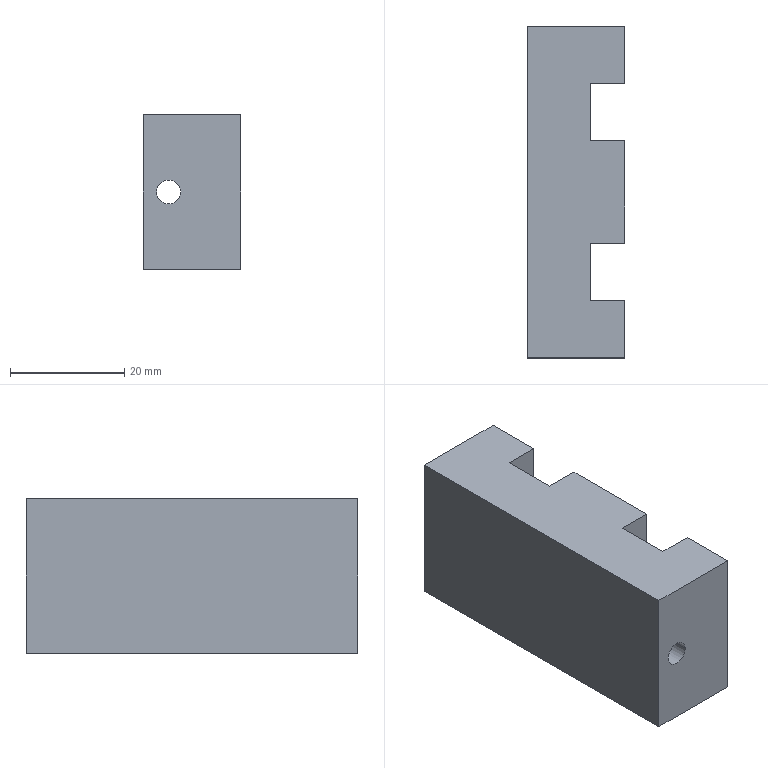Part | SolidWorks | features ICE 3, 3DProfileFeature 1, Extrusion 1, Fillet 1, HoleWzd 1 | 1 solid | 35 faces | box 17 x 58 x 27 mm | volume 21446 mm3 | plane 29 | cylinder 6 | commonest cylinder face diameters 2 x4 4.2 x2
STEP:
#1=CARTESIAN_POINT('',(2.3,-29.,0.));
#2=VERTEX_POINT('',#1);
#3=CARTESIAN_POINT('',(6.5,-29.,0.));
#4=VERTEX_POINT('',#3);
#5=CARTESIAN_POINT('',(4.4,-29.,0.));
#6=DIRECTION('',(0.,-1.,0.));
#7=DIRECTION('',(-1.,0.,0.));
#8=AXIS2_PLACEMENT_3D('',#5,#6,#7);
#9=CIRCLE('',#8,2.1);
#10=EDGE_CURVE('',#2,#4,#9,.T.);
#11=ORIENTED_EDGE('',*,*,#10,.T.);
#12=CARTESIAN_POINT('',(6.5,29.,0.));
#13=VERTEX_POINT('',#12);
#14=CARTESIAN_POINT('',(6.5,-34.94,0.));
#15=DIRECTION('',(0.,1.,0.));
#16=VECTOR('',#15,1000.);
#17=LINE('',#14,#16);
#18=EDGE_CURVE('',#4,#13,#17,.T.);
#19=ORIENTED_EDGE('',*,*,#18,.T.);
#20=CARTESIAN_POINT('',(2.3,29.,0.));
#21=VERTEX_POINT('',#20);
#22=CARTESIAN_POINT('',(4.4,29.,0.));
#23=DIRECTION('',(0.,1.,0.));
#24=DIRECTION('',(-1.,0.,0.));
#25=AXIS2_PLACEMENT_3D('',#22,#23,#24);
#26=CIRCLE('',#25,2.1);
#27=EDGE_CURVE('',#13,#21,#26,.T.);
#28=ORIENTED_EDGE('',*,*,#27,.T.);
#29=CARTESIAN_POINT('',(2.3,-34.94,0.));
#30=DIRECTION('',(0.,1.,0.));
#31=VECTOR('',#30,1000.);
#32=LINE('',#29,#31);
#33=EDGE_CURVE('',#2,#21,#32,.T.);
#34=ORIENTED_EDGE('',*,*,#33,.F.);
#35=EDGE_LOOP('',(#11,#19,#28,#34));
#36=FACE_OUTER_BOUND('',#35,.T.);
#37=CARTESIAN_POINT('',(4.4,-34.94,0.));
#38=DIRECTION('',(0.,1.,0.));
#39=DIRECTION('',(-1.,0.,0.));
#40=AXIS2_PLACEMENT_3D('',#37,#38,#39);
#41=CYLINDRICAL_SURFACE('',#40,2.1);
#42=ADVANCED_FACE('',(#36),#41,.F.);
#43=ORIENTED_EDGE('',*,*,#10,.F.);
#44=CARTESIAN_POINT('',(4.4,-29.,0.));
#45=DIRECTION('',(0.,-1.,0.));
#46=DIRECTION('',(-1.,0.,0.));
#47=AXIS2_PLACEMENT_3D('',#44,#45,#46);
#48=CIRCLE('',#47,2.1);
#49=EDGE_CURVE('',#4,#2,#48,.T.);
#50=ORIENTED_EDGE('',*,*,#49,.F.);
#51=EDGE_LOOP('',(#43,#50));
#52=FACE_BOUND('',#51,.T.);
#53=CARTESIAN_POINT('',(0.,-29.,-13.5));
#54=VERTEX_POINT('',#53);
#55=CARTESIAN_POINT('',(17.,-29.,-13.5));
#56=VERTEX_POINT('',#55);
#57=CARTESIAN_POINT('',(17.,-29.,-13.5));
#58=DIRECTION('',(1.,0.,0.));
#59=VECTOR('',#58,1000.);
#60=LINE('',#57,#59);
#61=EDGE_CURVE('',#54,#56,#60,.T.);
#62=ORIENTED_EDGE('',*,*,#61,.T.);
#63=CARTESIAN_POINT('',(17.,-29.,13.5));
#64=VERTEX_POINT('',#63);
#65=CARTESIAN_POINT('',(17.,-29.,13.5));
#66=DIRECTION('',(0.,0.,-1.));
#67=VECTOR('',#66,1000.);
#68=LINE('',#65,#67);
#69=EDGE_CURVE('',#64,#56,#68,.T.);
#70=ORIENTED_EDGE('',*,*,#69,.F.);
#71=CARTESIAN_POINT('',(0.,-29.,13.5));
#72=VERTEX_POINT('',#71);
#73=CARTESIAN_POINT('',(17.,-29.,13.5));
#74=DIRECTION('',(1.,0.,0.));
#75=VECTOR('',#74,1000.);
#76=LINE('',#73,#75);
#77=EDGE_CURVE('',#72,#64,#76,.T.);
#78=ORIENTED_EDGE('',*,*,#77,.F.);
#79=CARTESIAN_POINT('',(0.,-29.,13.5));
#80=DIRECTION('',(0.,0.,-1.));
#81=VECTOR('',#80,1000.);
#82=LINE('',#79,#81);
#83=EDGE_CURVE('',#72,#54,#82,.T.);
#84=ORIENTED_EDGE('',*,*,#83,.T.);
#85=EDGE_LOOP('',(#62,#70,#78,#84));
#86=FACE_OUTER_BOUND('',#85,.T.);
#87=CARTESIAN_POINT('',(17.,-29.,13.5));
#88=DIRECTION('',(0.,1.,0.));
#89=DIRECTION('',(-1.,0.,0.));
#90=AXIS2_PLACEMENT_3D('',#87,#88,#89);
#91=PLANE('',#90);
#92=ADVANCED_FACE('',(#52,#86),#91,.F.);
#93=CARTESIAN_POINT('',(17.,-27.,10.5));
#94=VERTEX_POINT('',#93);
#95=CARTESIAN_POINT('',(17.,-27.,-10.5));
#96=VERTEX_POINT('',#95);
#97=CARTESIAN_POINT('',(17.,-27.,10.5));
#98=DIRECTION('',(0.,0.,-1.));
#99=VECTOR('',#98,1000.);
#100=LINE('',#97,#99);
#101=EDGE_CURVE('',#94,#96,#100,.T.);
#102=ORIENTED_EDGE('',*,*,#101,.F.);
#103=CARTESIAN_POINT('',(17.,-21.,10.5));
#104=VERTEX_POINT('',#103);
#105=CARTESIAN_POINT('',(17.,-21.,10.5));
#106=DIRECTION('',(0.,-1.,0.));
#107=VECTOR('',#106,1000.);
#108=LINE('',#105,#107);
#109=EDGE_CURVE('',#104,#94,#108,.T.);
#110=ORIENTED_EDGE('',*,*,#109,.F.);
#111=CARTESIAN_POINT('',(17.,-21.,-10.5));
#112=VERTEX_POINT('',#111);
#113=CARTESIAN_POINT('',(17.,-21.,10.5));
#114=DIRECTION('',(0.,0.,1.));
#115=VECTOR('',#114,1000.);
#116=LINE('',#113,#115);
#117=EDGE_CURVE('',#112,#104,#116,.T.);
#118=ORIENTED_EDGE('',*,*,#117,.F.);
#119=CARTESIAN_POINT('',(17.,-21.,-10.5));
#120=DIRECTION('',(0.,1.,0.));
#121=VECTOR('',#120,1000.);
#122=LINE('',#119,#121);
#123=EDGE_CURVE('',#96,#112,#122,.T.);
#124=ORIENTED_EDGE('',*,*,#123,.F.);
#125=EDGE_LOOP('',(#102,#110,#118,#124));
#126=FACE_BOUND('',#125,.T.);
#127=CARTESIAN_POINT('',(17.,-19.,-13.5));
#128=VERTEX_POINT('',#127);
#129=CARTESIAN_POINT('',(17.,-19.,-13.5));
#130=DIRECTION('',(0.,1.,0.));
#131=VECTOR('',#130,1000.);
#132=LINE('',#129,#131);
#133=EDGE_CURVE('',#56,#128,#132,.T.);
#134=ORIENTED_EDGE('',*,*,#133,.T.);
#135=CARTESIAN_POINT('',(17.,-19.,13.5));
#136=VERTEX_POINT('',#135);
#137=CARTESIAN_POINT('',(17.,-19.,13.5));
#138=DIRECTION('',(0.,0.,-1.));
#139=VECTOR('',#138,1000.);
#140=LINE('',#137,#139);
#141=EDGE_CURVE('',#136,#128,#140,.T.);
#142=ORIENTED_EDGE('',*,*,#141,.F.);
#143=CARTESIAN_POINT('',(17.,-19.,13.5));
#144=DIRECTION('',(0.,1.,0.));
#145=VECTOR('',#144,1000.);
#146=LINE('',#143,#145);
#147=EDGE_CURVE('',#64,#136,#146,.T.);
#148=ORIENTED_EDGE('',*,*,#147,.F.);
#149=ORIENTED_EDGE('',*,*,#69,.T.);
#150=EDGE_LOOP('',(#134,#142,#148,#149));
#151=FACE_OUTER_BOUND('',#150,.T.);
#152=CARTESIAN_POINT('',(17.,-19.,13.5));
#153=DIRECTION('',(-1.,0.,0.));
#154=DIRECTION('',(0.,-1.,0.));
#155=AXIS2_PLACEMENT_3D('',#152,#153,#154);
#156=PLANE('',#155);
#157=ADVANCED_FACE('',(#126,#151),#156,.F.);
#158=CARTESIAN_POINT('',(11.,-19.,-13.5));
#159=VERTEX_POINT('',#158);
#160=CARTESIAN_POINT('',(11.,-19.,-13.5));
#161=DIRECTION('',(-1.,0.,0.));
#162=VECTOR('',#161,1000.);
#163=LINE('',#160,#162);
#164=EDGE_CURVE('',#128,#159,#163,.T.);
#165=ORIENTED_EDGE('',*,*,#164,.T.);
#166=CARTESIAN_POINT('',(11.,-19.,13.5));
#167=VERTEX_POINT('',#166);
#168=CARTESIAN_POINT('',(11.,-19.,13.5));
#169=DIRECTION('',(0.,0.,-1.));
#170=VECTOR('',#169,1000.);
#171=LINE('',#168,#170);
#172=EDGE_CURVE('',#167,#159,#171,.T.);
#173=ORIENTED_EDGE('',*,*,#172,.F.);
#174=CARTESIAN_POINT('',(11.,-19.,13.5));
#175=DIRECTION('',(-1.,0.,0.));
#176=VECTOR('',#175,1000.);
#177=LINE('',#174,#176);
#178=EDGE_CURVE('',#136,#167,#177,.T.);
#179=ORIENTED_EDGE('',*,*,#178,.F.);
#180=ORIENTED_EDGE('',*,*,#141,.T.);
#181=EDGE_LOOP('',(#165,#173,#179,#180));
#182=FACE_OUTER_BOUND('',#181,.T.);
#183=CARTESIAN_POINT('',(11.,-19.,13.5));
#184=DIRECTION('',(0.,-1.,0.));
#185=DIRECTION('',(0.,0.,-1.));
#186=AXIS2_PLACEMENT_3D('',#183,#184,#185);
#187=PLANE('',#186);
#188=ADVANCED_FACE('',(#182),#187,.F.);
#189=CARTESIAN_POINT('',(11.,-9.,-13.5));
#190=VERTEX_POINT('',#189);
#191=CARTESIAN_POINT('',(11.,-9.,-13.5));
#192=DIRECTION('',(0.,1.,0.));
#193=VECTOR('',#192,1000.);
#194=LINE('',#191,#193);
#195=EDGE_CURVE('',#159,#190,#194,.T.);
#196=ORIENTED_EDGE('',*,*,#195,.T.);
#197=CARTESIAN_POINT('',(11.,-9.,13.5));
#198=VERTEX_POINT('',#197);
#199=CARTESIAN_POINT('',(11.,-9.,13.5));
#200=DIRECTION('',(0.,0.,-1.));
#201=VECTOR('',#200,1000.);
#202=LINE('',#199,#201);
#203=EDGE_CURVE('',#198,#190,#202,.T.);
#204=ORIENTED_EDGE('',*,*,#203,.F.);
#205=CARTESIAN_POINT('',(11.,-9.,13.5));
#206=DIRECTION('',(0.,1.,0.));
#207=VECTOR('',#206,1000.);
#208=LINE('',#205,#207);
#209=EDGE_CURVE('',#167,#198,#208,.T.);
#210=ORIENTED_EDGE('',*,*,#209,.F.);
#211=ORIENTED_EDGE('',*,*,#172,.T.);
#212=EDGE_LOOP('',(#196,#204,#210,#211));
#213=FACE_OUTER_BOUND('',#212,.T.);
#214=CARTESIAN_POINT('',(11.,-9.,13.5));
#215=DIRECTION('',(-1.,0.,0.));
#216=DIRECTION('',(0.,-1.,0.));
#217=AXIS2_PLACEMENT_3D('',#214,#215,#216);
#218=PLANE('',#217);
#219=ADVANCED_FACE('',(#213),#218,.F.);
#220=CARTESIAN_POINT('',(17.,-9.,-13.5));
#221=VERTEX_POINT('',#220);
#222=CARTESIAN_POINT('',(17.,-9.,-13.5));
#223=DIRECTION('',(1.,0.,0.));
#224=VECTOR('',#223,1000.);
#225=LINE('',#222,#224);
#226=EDGE_CURVE('',#190,#221,#225,.T.);
#227=ORIENTED_EDGE('',*,*,#226,.T.);
#228=CARTESIAN_POINT('',(17.,-9.,13.5));
#229=VERTEX_POINT('',#228);
#230=CARTESIAN_POINT('',(17.,-9.,13.5));
#231=DIRECTION('',(0.,0.,-1.));
#232=VECTOR('',#231,1000.);
#233=LINE('',#230,#232);
#234=EDGE_CURVE('',#229,#221,#233,.T.);
#235=ORIENTED_EDGE('',*,*,#234,.F.);
#236=CARTESIAN_POINT('',(17.,-9.,13.5));
#237=DIRECTION('',(1.,0.,0.));
#238=VECTOR('',#237,1000.);
#239=LINE('',#236,#238);
#240=EDGE_CURVE('',#198,#229,#239,.T.);
#241=ORIENTED_EDGE('',*,*,#240,.F.);
#242=ORIENTED_EDGE('',*,*,#203,.T.);
#243=EDGE_LOOP('',(#227,#235,#241,#242));
#244=FACE_OUTER_BOUND('',#243,.T.);
#245=CARTESIAN_POINT('',(17.,-9.,13.5));
#246=DIRECTION('',(0.,1.,0.));
#247=DIRECTION('',(0.,0.,1.));
#248=AXIS2_PLACEMENT_3D('',#245,#246,#247);
#249=PLANE('',#248);
#250=ADVANCED_FACE('',(#244),#249,.F.);
#251=CARTESIAN_POINT('',(17.,7.5,-10.5));
#252=VERTEX_POINT('',#251);
#253=CARTESIAN_POINT('',(17.,7.5,10.5));
#254=VERTEX_POINT('',#253);
#255=CARTESIAN_POINT('',(17.,7.5,10.5));
#256=DIRECTION('',(0.,0.,1.));
#257=VECTOR('',#256,1000.);
#258=LINE('',#255,#257);
#259=EDGE_CURVE('',#252,#254,#258,.T.);
#260=ORIENTED_EDGE('',*,*,#259,.F.);
#261=CARTESIAN_POINT('',(17.,-7.5,-10.5));
#262=VERTEX_POINT('',#261);
#263=CARTESIAN_POINT('',(17.,-7.5,-10.5));
#264=DIRECTION('',(0.,1.,0.));
#265=VECTOR('',#264,1000.);
#266=LINE('',#263,#265);
#267=EDGE_CURVE('',#262,#252,#266,.T.);
#268=ORIENTED_EDGE('',*,*,#267,.F.);
#269=CARTESIAN_POINT('',(17.,-7.5,10.5));
#270=VERTEX_POINT('',#269);
#271=CARTESIAN_POINT('',(17.,-7.5,10.5));
#272=DIRECTION('',(0.,0.,-1.));
#273=VECTOR('',#272,1000.);
#274=LINE('',#271,#273);
#275=EDGE_CURVE('',#270,#262,#274,.T.);
#276=ORIENTED_EDGE('',*,*,#275,.F.);
#277=CARTESIAN_POINT('',(17.,-7.5,10.5));
#278=DIRECTION('',(0.,-1.,0.));
#279=VECTOR('',#278,1000.);
#280=LINE('',#277,#279);
#281=EDGE_CURVE('',#254,#270,#280,.T.);
#282=ORIENTED_EDGE('',*,*,#281,.F.);
#283=EDGE_LOOP('',(#260,#268,#276,#282));
#284=FACE_BOUND('',#283,.T.);
#285=CARTESIAN_POINT('',(17.,9.,-13.5));
#286=VERTEX_POINT('',#285);
#287=CARTESIAN_POINT('',(17.,9.,-13.5));
#288=DIRECTION('',(0.,1.,0.));
#289=VECTOR('',#288,1000.);
#290=LINE('',#287,#289);
#291=EDGE_CURVE('',#221,#286,#290,.T.);
#292=ORIENTED_EDGE('',*,*,#291,.T.);
#293=CARTESIAN_POINT('',(17.,9.,13.5));
#294=VERTEX_POINT('',#293);
#295=CARTESIAN_POINT('',(17.,9.,13.5));
#296=DIRECTION('',(0.,0.,-1.));
#297=VECTOR('',#296,1000.);
#298=LINE('',#295,#297);
#299=EDGE_CURVE('',#294,#286,#298,.T.);
#300=ORIENTED_EDGE('',*,*,#299,.F.);
#301=CARTESIAN_POINT('',(17.,9.,13.5));
#302=DIRECTION('',(0.,1.,0.));
#303=VECTOR('',#302,1000.);
#304=LINE('',#301,#303);
#305=EDGE_CURVE('',#229,#294,#304,.T.);
#306=ORIENTED_EDGE('',*,*,#305,.F.);
#307=ORIENTED_EDGE('',*,*,#234,.T.);
#308=EDGE_LOOP('',(#292,#300,#306,#307));
#309=FACE_OUTER_BOUND('',#308,.T.);
#310=CARTESIAN_POINT('',(17.,9.,13.5));
#311=DIRECTION('',(-1.,0.,0.));
#312=DIRECTION('',(0.,-1.,0.));
#313=AXIS2_PLACEMENT_3D('',#310,#311,#312);
#314=PLANE('',#313);
#315=ADVANCED_FACE('',(#284,#309),#314,.F.);
#316=CARTESIAN_POINT('',(11.,9.,-13.5));
#317=VERTEX_POINT('',#316);
#318=CARTESIAN_POINT('',(11.,9.,-13.5));
#319=DIRECTION('',(-1.,0.,0.));
#320=VECTOR('',#319,1000.);
#321=LINE('',#318,#320);
#322=EDGE_CURVE('',#286,#317,#321,.T.);
#323=ORIENTED_EDGE('',*,*,#322,.T.);
#324=CARTESIAN_POINT('',(11.,9.,13.5));
#325=VERTEX_POINT('',#324);
#326=CARTESIAN_POINT('',(11.,9.,13.5));
#327=DIRECTION('',(0.,0.,-1.));
#328=VECTOR('',#327,1000.);
#329=LINE('',#326,#328);
#330=EDGE_CURVE('',#325,#317,#329,.T.);
#331=ORIENTED_EDGE('',*,*,#330,.F.);
#332=CARTESIAN_POINT('',(11.,9.,13.5));
#333=DIRECTION('',(-1.,0.,0.));
#334=VECTOR('',#333,1000.);
#335=LINE('',#332,#334);
#336=EDGE_CURVE('',#294,#325,#335,.T.);
#337=ORIENTED_EDGE('',*,*,#336,.F.);
#338=ORIENTED_EDGE('',*,*,#299,.T.);
#339=EDGE_LOOP('',(#323,#331,#337,#338));
#340=FACE_OUTER_BOUND('',#339,.T.);
#341=CARTESIAN_POINT('',(11.,9.,13.5));
#342=DIRECTION('',(0.,-1.,0.));
#343=DIRECTION('',(0.,0.,-1.));
#344=AXIS2_PLACEMENT_3D('',#341,#342,#343);
#345=PLANE('',#344);
#346=ADVANCED_FACE('',(#340),#345,.F.);
#347=CARTESIAN_POINT('',(11.,19.,-13.5));
#348=VERTEX_POINT('',#347);
#349=CARTESIAN_POINT('',(11.,19.,-13.5));
#350=DIRECTION('',(0.,1.,0.));
#351=VECTOR('',#350,1000.);
#352=LINE('',#349,#351);
#353=EDGE_CURVE('',#317,#348,#352,.T.);
#354=ORIENTED_EDGE('',*,*,#353,.T.);
#355=CARTESIAN_POINT('',(11.,19.,13.5));
#356=VERTEX_POINT('',#355);
#357=CARTESIAN_POINT('',(11.,19.,13.5));
#358=DIRECTION('',(0.,0.,-1.));
#359=VECTOR('',#358,1000.);
#360=LINE('',#357,#359);
#361=EDGE_CURVE('',#356,#348,#360,.T.);
#362=ORIENTED_EDGE('',*,*,#361,.F.);
#363=CARTESIAN_POINT('',(11.,19.,13.5));
#364=DIRECTION('',(0.,1.,0.));
#365=VECTOR('',#364,1000.);
#366=LINE('',#363,#365);
#367=EDGE_CURVE('',#325,#356,#366,.T.);
#368=ORIENTED_EDGE('',*,*,#367,.F.);
#369=ORIENTED_EDGE('',*,*,#330,.T.);
#370=EDGE_LOOP('',(#354,#362,#368,#369));
#371=FACE_OUTER_BOUND('',#370,.T.);
#372=CARTESIAN_POINT('',(11.,19.,13.5));
#373=DIRECTION('',(-1.,0.,0.));
#374=DIRECTION('',(0.,-1.,0.));
#375=AXIS2_PLACEMENT_3D('',#372,#373,#374);
#376=PLANE('',#375);
#377=ADVANCED_FACE('',(#371),#376,.F.);
#378=CARTESIAN_POINT('',(17.,19.,-13.5));
#379=VERTEX_POINT('',#378);
#380=CARTESIAN_POINT('',(17.,19.,-13.5));
#381=DIRECTION('',(1.,0.,0.));
#382=VECTOR('',#381,1000.);
#383=LINE('',#380,#382);
#384=EDGE_CURVE('',#348,#379,#383,.T.);
#385=ORIENTED_EDGE('',*,*,#384,.T.);
#386=CARTESIAN_POINT('',(17.,19.,13.5));
#387=VERTEX_POINT('',#386);
#388=CARTESIAN_POINT('',(17.,19.,13.5));
#389=DIRECTION('',(0.,0.,-1.));
#390=VECTOR('',#389,1000.);
#391=LINE('',#388,#390);
#392=EDGE_CURVE('',#387,#379,#391,.T.);
#393=ORIENTED_EDGE('',*,*,#392,.F.);
#394=CARTESIAN_POINT('',(17.,19.,13.5));
#395=DIRECTION('',(1.,0.,0.));
#396=VECTOR('',#395,1000.);
#397=LINE('',#394,#396);
#398=EDGE_CURVE('',#356,#387,#397,.T.);
#399=ORIENTED_EDGE('',*,*,#398,.F.);
#400=ORIENTED_EDGE('',*,*,#361,.T.);
#401=EDGE_LOOP('',(#385,#393,#399,#400));
#402=FACE_OUTER_BOUND('',#401,.T.);
#403=CARTESIAN_POINT('',(17.,19.,13.5));
#404=DIRECTION('',(0.,1.,0.));
#405=DIRECTION('',(-1.,0.,0.));
#406=AXIS2_PLACEMENT_3D('',#403,#404,#405);
#407=PLANE('',#406);
#408=ADVANCED_FACE('',(#402),#407,.F.);
#409=CARTESIAN_POINT('',(17.,27.,-9.5));
#410=VERTEX_POINT('',#409);
#411=CARTESIAN_POINT('',(17.,27.,9.5));
#412=VERTEX_POINT('',#411);
#413=CARTESIAN_POINT('',(17.,27.,10.5));
#414=DIRECTION('',(0.,0.,1.));
#415=VECTOR('',#414,1000.);
#416=LINE('',#413,#415);
#417=EDGE_CURVE('',#410,#412,#416,.T.);
#418=ORIENTED_EDGE('',*,*,#417,.F.);
#419=CARTESIAN_POINT('',(17.,26.,-10.5));
#420=VERTEX_POINT('',#419);
#421=CARTESIAN_POINT('',(17.,26.,-9.5));
#422=DIRECTION('',(-1.,0.,0.));
#423=DIRECTION('',(0.,0.,1.));
#424=AXIS2_PLACEMENT_3D('',#421,#422,#423);
#425=CIRCLE('',#424,1.);
#426=EDGE_CURVE('',#410,#420,#425,.T.);
#427=ORIENTED_EDGE('',*,*,#426,.T.);
#428=CARTESIAN_POINT('',(17.,22.,-10.5));
#429=VERTEX_POINT('',#428);
#430=CARTESIAN_POINT('',(17.,21.,-10.5));
#431=DIRECTION('',(0.,1.,0.));
#432=VECTOR('',#431,1000.);
#433=LINE('',#430,#432);
#434=EDGE_CURVE('',#429,#420,#433,.T.);
#435=ORIENTED_EDGE('',*,*,#434,.F.);
#436=CARTESIAN_POINT('',(17.,21.,-9.5));
#437=VERTEX_POINT('',#436);
#438=CARTESIAN_POINT('',(17.,22.,-9.5));
#439=DIRECTION('',(-1.,0.,0.));
#440=DIRECTION('',(0.,0.,1.));
#441=AXIS2_PLACEMENT_3D('',#438,#439,#440);
#442=CIRCLE('',#441,1.);
#443=EDGE_CURVE('',#429,#437,#442,.T.);
#444=ORIENTED_EDGE('',*,*,#443,.T.);
#445=CARTESIAN_POINT('',(17.,21.,9.5));
#446=VERTEX_POINT('',#445);
#447=CARTESIAN_POINT('',(17.,21.,10.5));
#448=DIRECTION('',(0.,0.,-1.));
#449=VECTOR('',#448,1000.);
#450=LINE('',#447,#449);
#451=EDGE_CURVE('',#446,#437,#450,.T.);
#452=ORIENTED_EDGE('',*,*,#451,.F.);
#453=CARTESIAN_POINT('',(17.,22.,10.5));
#454=VERTEX_POINT('',#453);
#455=CARTESIAN_POINT('',(17.,22.,9.5));
#456=DIRECTION('',(-1.,0.,0.));
#457=DIRECTION('',(0.,0.,1.));
#458=AXIS2_PLACEMENT_3D('',#455,#456,#457);
#459=CIRCLE('',#458,1.);
#460=EDGE_CURVE('',#446,#454,#459,.T.);
#461=ORIENTED_EDGE('',*,*,#460,.T.);
#462=CARTESIAN_POINT('',(17.,26.,10.5));
#463=VERTEX_POINT('',#462);
#464=CARTESIAN_POINT('',(17.,21.,10.5));
#465=DIRECTION('',(0.,-1.,0.));
#466=VECTOR('',#465,1000.);
#467=LINE('',#464,#466);
#468=EDGE_CURVE('',#463,#454,#467,.T.);
#469=ORIENTED_EDGE('',*,*,#468,.F.);
#470=CARTESIAN_POINT('',(17.,26.,9.5));
#471=DIRECTION('',(-1.,0.,0.));
#472=DIRECTION('',(0.,0.,1.));
#473=AXIS2_PLACEMENT_3D('',#470,#471,#472);
#474=CIRCLE('',#473,1.);
#475=EDGE_CURVE('',#463,#412,#474,.T.);
#476=ORIENTED_EDGE('',*,*,#475,.T.);
#477=EDGE_LOOP('',(#418,#427,#435,#444,#452,#461,#469,#476));
#478=FACE_BOUND('',#477,.T.);
#479=CARTESIAN_POINT('',(17.,29.,-13.5));
#480=VERTEX_POINT('',#479);
#481=CARTESIAN_POINT('',(17.,29.,-13.5));
#482=DIRECTION('',(0.,1.,0.));
#483=VECTOR('',#482,1000.);
#484=LINE('',#481,#483);
#485=EDGE_CURVE('',#379,#480,#484,.T.);
#486=ORIENTED_EDGE('',*,*,#485,.T.);
#487=CARTESIAN_POINT('',(17.,29.,13.5));
#488=VERTEX_POINT('',#487);
#489=CARTESIAN_POINT('',(17.,29.,13.5));
#490=DIRECTION('',(0.,0.,-1.));
#491=VECTOR('',#490,1000.);
#492=LINE('',#489,#491);
#493=EDGE_CURVE('',#488,#480,#492,.T.);
#494=ORIENTED_EDGE('',*,*,#493,.F.);
#495=CARTESIAN_POINT('',(17.,29.,13.5));
#496=DIRECTION('',(0.,1.,0.));
#497=VECTOR('',#496,1000.);
#498=LINE('',#495,#497);
#499=EDGE_CURVE('',#387,#488,#498,.T.);
#500=ORIENTED_EDGE('',*,*,#499,.F.);
#501=ORIENTED_EDGE('',*,*,#392,.T.);
#502=EDGE_LOOP('',(#486,#494,#500,#501));
#503=FACE_OUTER_BOUND('',#502,.T.);
#504=CARTESIAN_POINT('',(17.,29.,13.5));
#505=DIRECTION('',(-1.,0.,0.));
#506=DIRECTION('',(0.,0.,1.));
#507=AXIS2_PLACEMENT_3D('',#504,#505,#506);
#508=PLANE('',#507);
#509=ADVANCED_FACE('',(#478,#503),#508,.F.);
#510=CARTESIAN_POINT('',(4.4,29.,0.));
#511=DIRECTION('',(0.,1.,0.));
#512=DIRECTION('',(-1.,0.,0.));
#513=AXIS2_PLACEMENT_3D('',#510,#511,#512);
#514=CIRCLE('',#513,2.1);
#515=EDGE_CURVE('',#21,#13,#514,.T.);
#516=ORIENTED_EDGE('',*,*,#515,.F.);
#517=ORIENTED_EDGE('',*,*,#27,.F.);
#518=EDGE_LOOP('',(#516,#517));
#519=FACE_BOUND('',#518,.T.);
#520=CARTESIAN_POINT('',(0.,29.,-13.5));
#521=VERTEX_POINT('',#520);
#522=CARTESIAN_POINT('',(0.,29.,-13.5));
#523=DIRECTION('',(-1.,0.,0.));
#524=VECTOR('',#523,1000.);
#525=LINE('',#522,#524);
#526=EDGE_CURVE('',#480,#521,#525,.T.);
#527=ORIENTED_EDGE('',*,*,#526,.T.);
#528=CARTESIAN_POINT('',(0.,29.,13.5));
#529=VERTEX_POINT('',#528);
#530=CARTESIAN_POINT('',(0.,29.,13.5));
#531=DIRECTION('',(0.,0.,-1.));
#532=VECTOR('',#531,1000.);
#533=LINE('',#530,#532);
#534=EDGE_CURVE('',#529,#521,#533,.T.);
#535=ORIENTED_EDGE('',*,*,#534,.F.);
#536=CARTESIAN_POINT('',(0.,29.,13.5));
#537=DIRECTION('',(-1.,0.,0.));
#538=VECTOR('',#537,1000.);
#539=LINE('',#536,#538);
#540=EDGE_CURVE('',#488,#529,#539,.T.);
#541=ORIENTED_EDGE('',*,*,#540,.F.);
#542=ORIENTED_EDGE('',*,*,#493,.T.);
#543=EDGE_LOOP('',(#527,#535,#541,#542));
#544=FACE_OUTER_BOUND('',#543,.T.);
#545=CARTESIAN_POINT('',(0.,29.,13.5));
#546=DIRECTION('',(0.,-1.,0.));
#547=DIRECTION('',(0.,0.,-1.));
#548=AXIS2_PLACEMENT_3D('',#545,#546,#547);
#549=PLANE('',#548);
#550=ADVANCED_FACE('',(#519,#544),#549,.F.);
#551=CARTESIAN_POINT('',(0.,0.,-13.5));
#552=DIRECTION('',(0.,-1.,0.));
#553=VECTOR('',#552,1000.);
#554=LINE('',#551,#553);
#555=EDGE_CURVE('',#521,#54,#554,.T.);
#556=ORIENTED_EDGE('',*,*,#555,.T.);
#557=ORIENTED_EDGE('',*,*,#83,.F.);
#558=CARTESIAN_POINT('',(0.,-29.,13.5));
#559=DIRECTION('',(0.,-1.,0.));
#560=VECTOR('',#559,1000.);
#561=LINE('',#558,#560);
#562=EDGE_CURVE('',#529,#72,#561,.T.);
#563=ORIENTED_EDGE('',*,*,#562,.F.);
#564=ORIENTED_EDGE('',*,*,#534,.T.);
#565=EDGE_LOOP('',(#556,#557,#563,#564));
#566=FACE_OUTER_BOUND('',#565,.T.);
#567=CARTESIAN_POINT('',(0.,0.,13.5));
#568=DIRECTION('',(1.,0.,0.));
#569=DIRECTION('',(0.,0.,-1.));
#570=AXIS2_PLACEMENT_3D('',#567,#568,#569);
#571=PLANE('',#570);
#572=ADVANCED_FACE('',(#566),#571,.F.);
#573=ORIENTED_EDGE('',*,*,#562,.T.);
#574=ORIENTED_EDGE('',*,*,#77,.T.);
#575=ORIENTED_EDGE('',*,*,#147,.T.);
#576=ORIENTED_EDGE('',*,*,#178,.T.);
#577=ORIENTED_EDGE('',*,*,#209,.T.);
#578=ORIENTED_EDGE('',*,*,#240,.T.);
#579=ORIENTED_EDGE('',*,*,#305,.T.);
#580=ORIENTED_EDGE('',*,*,#336,.T.);
#581=ORIENTED_EDGE('',*,*,#367,.T.);
#582=ORIENTED_EDGE('',*,*,#398,.T.);
#583=ORIENTED_EDGE('',*,*,#499,.T.);
#584=ORIENTED_EDGE('',*,*,#540,.T.);
#585=EDGE_LOOP('',(#573,#574,#575,#576,#577,#578,#579,#580,#581,#582,#583,#584));
#586=FACE_OUTER_BOUND('',#585,.T.);
#587=CARTESIAN_POINT('',(0.,0.,13.5));
#588=DIRECTION('',(0.,0.,-1.));
#589=DIRECTION('',(-1.,0.,0.));
#590=AXIS2_PLACEMENT_3D('',#587,#588,#589);
#591=PLANE('',#590);
#592=ADVANCED_FACE('',(#586),#591,.F.);
#593=ORIENTED_EDGE('',*,*,#61,.F.);
#594=ORIENTED_EDGE('',*,*,#555,.F.);
#595=ORIENTED_EDGE('',*,*,#526,.F.);
#596=ORIENTED_EDGE('',*,*,#485,.F.);
#597=ORIENTED_EDGE('',*,*,#384,.F.);
#598=ORIENTED_EDGE('',*,*,#353,.F.);
#599=ORIENTED_EDGE('',*,*,#322,.F.);
#600=ORIENTED_EDGE('',*,*,#291,.F.);
#601=ORIENTED_EDGE('',*,*,#226,.F.);
#602=ORIENTED_EDGE('',*,*,#195,.F.);
#603=ORIENTED_EDGE('',*,*,#164,.F.);
#604=ORIENTED_EDGE('',*,*,#133,.F.);
#605=EDGE_LOOP('',(#593,#594,#595,#596,#597,#598,#599,#600,#601,#602,#603,#604));
#606=FACE_OUTER_BOUND('',#605,.T.);
#607=CARTESIAN_POINT('',(0.,0.,-13.5));
#608=DIRECTION('',(0.,0.,-1.));
#609=DIRECTION('',(-1.,0.,0.));
#610=AXIS2_PLACEMENT_3D('',#607,#608,#609);
#611=PLANE('',#610);
#612=ADVANCED_FACE('',(#606),#611,.T.);
#613=CARTESIAN_POINT('',(15.,22.,-10.5));
#614=VERTEX_POINT('',#613);
#615=CARTESIAN_POINT('',(15.,26.,-10.5));
#616=VERTEX_POINT('',#615);
#617=CARTESIAN_POINT('',(15.,21.,-10.5));
#618=DIRECTION('',(0.,1.,0.));
#619=VECTOR('',#618,1000.);
#620=LINE('',#617,#619);
#621=EDGE_CURVE('',#614,#616,#620,.T.);
#622=ORIENTED_EDGE('',*,*,#621,.F.);
#623=CARTESIAN_POINT('',(17.,22.,-10.5));
#624=DIRECTION('',(1.,0.,0.));
#625=VECTOR('',#624,1000.);
#626=LINE('',#623,#625);
#627=EDGE_CURVE('',#614,#429,#626,.T.);
#628=ORIENTED_EDGE('',*,*,#627,.T.);
#629=ORIENTED_EDGE('',*,*,#434,.T.);
#630=CARTESIAN_POINT('',(15.,26.,-10.5));
#631=DIRECTION('',(-1.,0.,0.));
#632=VECTOR('',#631,1000.);
#633=LINE('',#630,#632);
#634=EDGE_CURVE('',#420,#616,#633,.T.);
#635=ORIENTED_EDGE('',*,*,#634,.T.);
#636=EDGE_LOOP('',(#622,#628,#629,#635));
#637=FACE_OUTER_BOUND('',#636,.T.);
#638=CARTESIAN_POINT('',(15.,21.,-10.5));
#639=DIRECTION('',(0.,0.,-1.));
#640=DIRECTION('',(-1.,0.,0.));
#641=AXIS2_PLACEMENT_3D('',#638,#639,#640);
#642=PLANE('',#641);
#643=ADVANCED_FACE('',(#637),#642,.F.);
#644=CARTESIAN_POINT('',(15.,21.,9.5));
#645=VERTEX_POINT('',#644);
#646=CARTESIAN_POINT('',(15.,21.,-9.5));
#647=VERTEX_POINT('',#646);
#648=CARTESIAN_POINT('',(15.,21.,10.5));
#649=DIRECTION('',(0.,0.,-1.));
#650=VECTOR('',#649,1000.);
#651=LINE('',#648,#650);
#652=EDGE_CURVE('',#645,#647,#651,.T.);
#653=ORIENTED_EDGE('',*,*,#652,.F.);
#654=CARTESIAN_POINT('',(17.,21.,9.5));
#655=DIRECTION('',(1.,0.,0.));
#656=VECTOR('',#655,1000.);
#657=LINE('',#654,#656);
#658=EDGE_CURVE('',#645,#446,#657,.T.);
#659=ORIENTED_EDGE('',*,*,#658,.T.);
#660=ORIENTED_EDGE('',*,*,#451,.T.);
#661=CARTESIAN_POINT('',(15.,21.,-9.5));
#662=DIRECTION('',(-1.,0.,0.));
#663=VECTOR('',#662,1000.);
#664=LINE('',#661,#663);
#665=EDGE_CURVE('',#437,#647,#664,.T.);
#666=ORIENTED_EDGE('',*,*,#665,.T.);
#667=EDGE_LOOP('',(#653,#659,#660,#666));
#668=FACE_OUTER_BOUND('',#667,.T.);
#669=CARTESIAN_POINT('',(15.,21.,10.5));
#670=DIRECTION('',(0.,-1.,0.));
#671=DIRECTION('',(0.,0.,-1.));
#672=AXIS2_PLACEMENT_3D('',#669,#670,#671);
#673=PLANE('',#672);
#674=ADVANCED_FACE('',(#668),#673,.F.);
#675=CARTESIAN_POINT('',(15.,26.,10.5));
#676=VERTEX_POINT('',#675);
#677=CARTESIAN_POINT('',(15.,22.,10.5));
#678=VERTEX_POINT('',#677);
#679=CARTESIAN_POINT('',(15.,21.,10.5));
#680=DIRECTION('',(0.,-1.,0.));
#681=VECTOR('',#680,1000.);
#682=LINE('',#679,#681);
#683=EDGE_CURVE('',#676,#678,#682,.T.);
#684=ORIENTED_EDGE('',*,*,#683,.F.);
#685=CARTESIAN_POINT('',(17.,26.,10.5));
#686=DIRECTION('',(1.,0.,0.));
#687=VECTOR('',#686,1000.);
#688=LINE('',#685,#687);
#689=EDGE_CURVE('',#676,#463,#688,.T.);
#690=ORIENTED_EDGE('',*,*,#689,.T.);
#691=ORIENTED_EDGE('',*,*,#468,.T.);
#692=CARTESIAN_POINT('',(15.,22.,10.5));
#693=DIRECTION('',(-1.,0.,0.));
#694=VECTOR('',#693,1000.);
#695=LINE('',#692,#694);
#696=EDGE_CURVE('',#454,#678,#695,.T.);
#697=ORIENTED_EDGE('',*,*,#696,.T.);
#698=EDGE_LOOP('',(#684,#690,#691,#697));
#699=FACE_OUTER_BOUND('',#698,.T.);
#700=CARTESIAN_POINT('',(15.,21.,10.5));
#701=DIRECTION('',(0.,0.,1.));
#702=DIRECTION('',(1.,0.,0.));
#703=AXIS2_PLACEMENT_3D('',#700,#701,#702);
#704=PLANE('',#703);
#705=ADVANCED_FACE('',(#699),#704,.F.);
#706=ORIENTED_EDGE('',*,*,#417,.T.);
#707=CARTESIAN_POINT('',(15.,27.,9.5));
#708=VERTEX_POINT('',#707);
#709=CARTESIAN_POINT('',(15.,27.,9.5));
#710=DIRECTION('',(-1.,0.,0.));
#711=VECTOR('',#710,1000.);
#712=LINE('',#709,#711);
#713=EDGE_CURVE('',#412,#708,#712,.T.);
#714=ORIENTED_EDGE('',*,*,#713,.T.);
#715=CARTESIAN_POINT('',(15.,27.,-9.5));
#716=VERTEX_POINT('',#715);
#717=CARTESIAN_POINT('',(15.,27.,10.5));
#718=DIRECTION('',(0.,0.,1.));
#719=VECTOR('',#718,1000.);
#720=LINE('',#717,#719);
#721=EDGE_CURVE('',#716,#708,#720,.T.);
#722=ORIENTED_EDGE('',*,*,#721,.F.);
#723=CARTESIAN_POINT('',(17.,27.,-9.5));
#724=DIRECTION('',(1.,0.,0.));
#725=VECTOR('',#724,1000.);
#726=LINE('',#723,#725);
#727=EDGE_CURVE('',#716,#410,#726,.T.);
#728=ORIENTED_EDGE('',*,*,#727,.T.);
#729=EDGE_LOOP('',(#706,#714,#722,#728));
#730=FACE_OUTER_BOUND('',#729,.T.);
#731=CARTESIAN_POINT('',(15.,27.,10.5));
#732=DIRECTION('',(0.,1.,0.));
#733=DIRECTION('',(0.,0.,1.));
#734=AXIS2_PLACEMENT_3D('',#731,#732,#733);
#735=PLANE('',#734);
#736=ADVANCED_FACE('',(#730),#735,.F.);
#737=ORIENTED_EDGE('',*,*,#721,.T.);
#738=CARTESIAN_POINT('',(15.,26.,9.5));
#739=DIRECTION('',(1.,0.,0.));
#740=DIRECTION('',(0.,0.,1.));
#741=AXIS2_PLACEMENT_3D('',#738,#739,#740);
#742=CIRCLE('',#741,1.);
#743=EDGE_CURVE('',#708,#676,#742,.T.);
#744=ORIENTED_EDGE('',*,*,#743,.T.);
#745=ORIENTED_EDGE('',*,*,#683,.T.);
#746=CARTESIAN_POINT('',(15.,22.,9.5));
#747=DIRECTION('',(1.,0.,0.));
#748=DIRECTION('',(0.,0.,1.));
#749=AXIS2_PLACEMENT_3D('',#746,#747,#748);
#750=CIRCLE('',#749,1.);
#751=EDGE_CURVE('',#678,#645,#750,.T.);
#752=ORIENTED_EDGE('',*,*,#751,.T.);
#753=ORIENTED_EDGE('',*,*,#652,.T.);
#754=CARTESIAN_POINT('',(15.,22.,-9.5));
#755=DIRECTION('',(1.,0.,0.));
#756=DIRECTION('',(0.,0.,1.));
#757=AXIS2_PLACEMENT_3D('',#754,#755,#756);
#758=CIRCLE('',#757,1.);
#759=EDGE_CURVE('',#647,#614,#758,.T.);
#760=ORIENTED_EDGE('',*,*,#759,.T.);
#761=ORIENTED_EDGE('',*,*,#621,.T.);
#762=CARTESIAN_POINT('',(15.,26.,-9.5));
#763=DIRECTION('',(1.,0.,0.));
#764=DIRECTION('',(0.,0.,1.));
#765=AXIS2_PLACEMENT_3D('',#762,#763,#764);
#766=CIRCLE('',#765,1.);
#767=EDGE_CURVE('',#616,#716,#766,.T.);
#768=ORIENTED_EDGE('',*,*,#767,.T.);
#769=EDGE_LOOP('',(#737,#744,#745,#752,#753,#760,#761,#768));
#770=FACE_OUTER_BOUND('',#769,.T.);
#771=CARTESIAN_POINT('',(15.,0.,0.));
#772=DIRECTION('',(-1.,0.,0.));
#773=DIRECTION('',(0.,0.,1.));
#774=AXIS2_PLACEMENT_3D('',#771,#772,#773);
#775=PLANE('',#774);
#776=ADVANCED_FACE('',(#770),#775,.F.);
#777=ORIENTED_EDGE('',*,*,#267,.T.);
#778=CARTESIAN_POINT('',(15.,7.5,-10.5));
#779=VERTEX_POINT('',#778);
#780=CARTESIAN_POINT('',(15.,7.5,-10.5));
#781=DIRECTION('',(1.,0.,0.));
#782=VECTOR('',#781,1000.);
#783=LINE('',#780,#782);
#784=EDGE_CURVE('',#779,#252,#783,.T.);
#785=ORIENTED_EDGE('',*,*,#784,.F.);
#786=CARTESIAN_POINT('',(15.,-7.5,-10.5));
#787=VERTEX_POINT('',#786);
#788=CARTESIAN_POINT('',(15.,-7.5,-10.5));
#789=DIRECTION('',(0.,1.,0.));
#790=VECTOR('',#789,1000.);
#791=LINE('',#788,#790);
#792=EDGE_CURVE('',#787,#779,#791,.T.);
#793=ORIENTED_EDGE('',*,*,#792,.F.);
#794=CARTESIAN_POINT('',(15.,-7.5,-10.5));
#795=DIRECTION('',(1.,0.,0.));
#796=VECTOR('',#795,1000.);
#797=LINE('',#794,#796);
#798=EDGE_CURVE('',#787,#262,#797,.T.);
#799=ORIENTED_EDGE('',*,*,#798,.T.);
#800=EDGE_LOOP('',(#777,#785,#793,#799));
#801=FACE_OUTER_BOUND('',#800,.T.);
#802=CARTESIAN_POINT('',(15.,-7.5,-10.5));
#803=DIRECTION('',(0.,0.,-1.));
#804=DIRECTION('',(-1.,0.,0.));
#805=AXIS2_PLACEMENT_3D('',#802,#803,#804);
#806=PLANE('',#805);
#807=ADVANCED_FACE('',(#801),#806,.F.);
#808=ORIENTED_EDGE('',*,*,#275,.T.);
#809=ORIENTED_EDGE('',*,*,#798,.F.);
#810=CARTESIAN_POINT('',(15.,-7.5,10.5));
#811=VERTEX_POINT('',#810);
#812=CARTESIAN_POINT('',(15.,-7.5,10.5));
#813=DIRECTION('',(0.,0.,-1.));
#814=VECTOR('',#813,1000.);
#815=LINE('',#812,#814);
#816=EDGE_CURVE('',#811,#787,#815,.T.);
#817=ORIENTED_EDGE('',*,*,#816,.F.);
#818=CARTESIAN_POINT('',(15.,-7.5,10.5));
#819=DIRECTION('',(1.,0.,0.));
#820=VECTOR('',#819,1000.);
#821=LINE('',#818,#820);
#822=EDGE_CURVE('',#811,#270,#821,.T.);
#823=ORIENTED_EDGE('',*,*,#822,.T.);
#824=EDGE_LOOP('',(#808,#809,#817,#823));
#825=FACE_OUTER_BOUND('',#824,.T.);
#826=CARTESIAN_POINT('',(15.,-7.5,10.5));
#827=DIRECTION('',(0.,-1.,0.));
#828=DIRECTION('',(0.,0.,-1.));
#829=AXIS2_PLACEMENT_3D('',#826,#827,#828);
#830=PLANE('',#829);
#831=ADVANCED_FACE('',(#825),#830,.F.);
#832=ORIENTED_EDGE('',*,*,#281,.T.);
#833=ORIENTED_EDGE('',*,*,#822,.F.);
#834=CARTESIAN_POINT('',(15.,7.5,10.5));
#835=VERTEX_POINT('',#834);
#836=CARTESIAN_POINT('',(15.,-7.5,10.5));
#837=DIRECTION('',(0.,-1.,0.));
#838=VECTOR('',#837,1000.);
#839=LINE('',#836,#838);
#840=EDGE_CURVE('',#835,#811,#839,.T.);
#841=ORIENTED_EDGE('',*,*,#840,.F.);
#842=CARTESIAN_POINT('',(15.,7.5,10.5));
#843=DIRECTION('',(1.,0.,0.));
#844=VECTOR('',#843,1000.);
#845=LINE('',#842,#844);
#846=EDGE_CURVE('',#835,#254,#845,.T.);
#847=ORIENTED_EDGE('',*,*,#846,.T.);
#848=EDGE_LOOP('',(#832,#833,#841,#847));
#849=FACE_OUTER_BOUND('',#848,.T.);
#850=CARTESIAN_POINT('',(15.,-7.5,10.5));
#851=DIRECTION('',(0.,0.,1.));
#852=DIRECTION('',(1.,0.,0.));
#853=AXIS2_PLACEMENT_3D('',#850,#851,#852);
#854=PLANE('',#853);
#855=ADVANCED_FACE('',(#849),#854,.F.);
#856=ORIENTED_EDGE('',*,*,#259,.T.);
#857=ORIENTED_EDGE('',*,*,#846,.F.);
#858=CARTESIAN_POINT('',(15.,7.5,10.5));
#859=DIRECTION('',(0.,0.,1.));
#860=VECTOR('',#859,1000.);
#861=LINE('',#858,#860);
#862=EDGE_CURVE('',#779,#835,#861,.T.);
#863=ORIENTED_EDGE('',*,*,#862,.F.);
#864=ORIENTED_EDGE('',*,*,#784,.T.);
#865=EDGE_LOOP('',(#856,#857,#863,#864));
#866=FACE_OUTER_BOUND('',#865,.T.);
#867=CARTESIAN_POINT('',(15.,7.5,10.5));
#868=DIRECTION('',(0.,1.,0.));
#869=DIRECTION('',(0.,0.,1.));
#870=AXIS2_PLACEMENT_3D('',#867,#868,#869);
#871=PLANE('',#870);
#872=ADVANCED_FACE('',(#866),#871,.F.);
#873=ORIENTED_EDGE('',*,*,#792,.T.);
#874=ORIENTED_EDGE('',*,*,#862,.T.);
#875=ORIENTED_EDGE('',*,*,#840,.T.);
#876=ORIENTED_EDGE('',*,*,#816,.T.);
#877=EDGE_LOOP('',(#873,#874,#875,#876));
#878=FACE_OUTER_BOUND('',#877,.T.);
#879=CARTESIAN_POINT('',(15.,0.,0.));
#880=DIRECTION('',(-1.,0.,0.));
#881=DIRECTION('',(0.,0.,1.));
#882=AXIS2_PLACEMENT_3D('',#879,#880,#881);
#883=PLANE('',#882);
#884=ADVANCED_FACE('',(#878),#883,.F.);
#885=ORIENTED_EDGE('',*,*,#109,.T.);
#886=CARTESIAN_POINT('',(15.,-27.,10.5));
#887=VERTEX_POINT('',#886);
#888=CARTESIAN_POINT('',(15.,-27.,10.5));
#889=DIRECTION('',(1.,0.,0.));
#890=VECTOR('',#889,1000.);
#891=LINE('',#888,#890);
#892=EDGE_CURVE('',#887,#94,#891,.T.);
#893=ORIENTED_EDGE('',*,*,#892,.F.);
#894=CARTESIAN_POINT('',(15.,-21.,10.5));
#895=VERTEX_POINT('',#894);
#896=CARTESIAN_POINT('',(15.,-21.,10.5));
#897=DIRECTION('',(0.,-1.,0.));
#898=VECTOR('',#897,1000.);
#899=LINE('',#896,#898);
#900=EDGE_CURVE('',#895,#887,#899,.T.);
#901=ORIENTED_EDGE('',*,*,#900,.F.);
#902=CARTESIAN_POINT('',(15.,-21.,10.5));
#903=DIRECTION('',(1.,0.,0.));
#904=VECTOR('',#903,1000.);
#905=LINE('',#902,#904);
#906=EDGE_CURVE('',#895,#104,#905,.T.);
#907=ORIENTED_EDGE('',*,*,#906,.T.);
#908=EDGE_LOOP('',(#885,#893,#901,#907));
#909=FACE_OUTER_BOUND('',#908,.T.);
#910=CARTESIAN_POINT('',(15.,-21.,10.5));
#911=DIRECTION('',(0.,0.,1.));
#912=DIRECTION('',(0.,-1.,0.));
#913=AXIS2_PLACEMENT_3D('',#910,#911,#912);
#914=PLANE('',#913);
#915=ADVANCED_FACE('',(#909),#914,.F.);
#916=ORIENTED_EDGE('',*,*,#117,.T.);
#917=ORIENTED_EDGE('',*,*,#906,.F.);
#918=CARTESIAN_POINT('',(15.,-21.,-10.5));
#919=VERTEX_POINT('',#918);
#920=CARTESIAN_POINT('',(15.,-21.,10.5));
#921=DIRECTION('',(0.,0.,1.));
#922=VECTOR('',#921,1000.);
#923=LINE('',#920,#922);
#924=EDGE_CURVE('',#919,#895,#923,.T.);
#925=ORIENTED_EDGE('',*,*,#924,.F.);
#926=CARTESIAN_POINT('',(15.,-21.,-10.5));
#927=DIRECTION('',(1.,0.,0.));
#928=VECTOR('',#927,1000.);
#929=LINE('',#926,#928);
#930=EDGE_CURVE('',#919,#112,#929,.T.);
#931=ORIENTED_EDGE('',*,*,#930,.T.);
#932=EDGE_LOOP('',(#916,#917,#925,#931));
#933=FACE_OUTER_BOUND('',#932,.T.);
#934=CARTESIAN_POINT('',(15.,-21.,10.5));
#935=DIRECTION('',(0.,1.,0.));
#936=DIRECTION('',(0.,0.,1.));
#937=AXIS2_PLACEMENT_3D('',#934,#935,#936);
#938=PLANE('',#937);
#939=ADVANCED_FACE('',(#933),#938,.F.);
#940=ORIENTED_EDGE('',*,*,#123,.T.);
#941=ORIENTED_EDGE('',*,*,#930,.F.);
#942=CARTESIAN_POINT('',(15.,-27.,-10.5));
#943=VERTEX_POINT('',#942);
#944=CARTESIAN_POINT('',(15.,-21.,-10.5));
#945=DIRECTION('',(0.,1.,0.));
#946=VECTOR('',#945,1000.);
#947=LINE('',#944,#946);
#948=EDGE_CURVE('',#943,#919,#947,.T.);
#949=ORIENTED_EDGE('',*,*,#948,.F.);
#950=CARTESIAN_POINT('',(15.,-27.,-10.5));
#951=DIRECTION('',(1.,0.,0.));
#952=VECTOR('',#951,1000.);
#953=LINE('',#950,#952);
#954=EDGE_CURVE('',#943,#96,#953,.T.);
#955=ORIENTED_EDGE('',*,*,#954,.T.);
#956=EDGE_LOOP('',(#940,#941,#949,#955));
#957=FACE_OUTER_BOUND('',#956,.T.);
#958=CARTESIAN_POINT('',(15.,-21.,-10.5));
#959=DIRECTION('',(0.,0.,-1.));
#960=DIRECTION('',(0.,1.,0.));
#961=AXIS2_PLACEMENT_3D('',#958,#959,#960);
#962=PLANE('',#961);
#963=ADVANCED_FACE('',(#957),#962,.F.);
#964=ORIENTED_EDGE('',*,*,#101,.T.);
#965=ORIENTED_EDGE('',*,*,#954,.F.);
#966=CARTESIAN_POINT('',(15.,-27.,10.5));
#967=DIRECTION('',(0.,0.,-1.));
#968=VECTOR('',#967,1000.);
#969=LINE('',#966,#968);
#970=EDGE_CURVE('',#887,#943,#969,.T.);
#971=ORIENTED_EDGE('',*,*,#970,.F.);
#972=ORIENTED_EDGE('',*,*,#892,.T.);
#973=EDGE_LOOP('',(#964,#965,#971,#972));
#974=FACE_OUTER_BOUND('',#973,.T.);
#975=CARTESIAN_POINT('',(15.,-27.,10.5));
#976=DIRECTION('',(0.,-1.,0.));
#977=DIRECTION('',(0.,0.,-1.));
#978=AXIS2_PLACEMENT_3D('',#975,#976,#977);
#979=PLANE('',#978);
#980=ADVANCED_FACE('',(#974),#979,.F.);
#981=ORIENTED_EDGE('',*,*,#900,.T.);
#982=ORIENTED_EDGE('',*,*,#970,.T.);
#983=ORIENTED_EDGE('',*,*,#948,.T.);
#984=ORIENTED_EDGE('',*,*,#924,.T.);
#985=EDGE_LOOP('',(#981,#982,#983,#984));
#986=FACE_OUTER_BOUND('',#985,.T.);
#987=CARTESIAN_POINT('',(15.,0.,0.));
#988=DIRECTION('',(1.,0.,0.));
#989=DIRECTION('',(0.,0.,-1.));
#990=AXIS2_PLACEMENT_3D('',#987,#988,#989);
#991=PLANE('',#990);
#992=ADVANCED_FACE('',(#986),#991,.T.);
#993=ORIENTED_EDGE('',*,*,#743,.F.);
#994=ORIENTED_EDGE('',*,*,#713,.F.);
#995=ORIENTED_EDGE('',*,*,#475,.F.);
#996=ORIENTED_EDGE('',*,*,#689,.F.);
#997=EDGE_LOOP('',(#993,#994,#995,#996));
#998=FACE_OUTER_BOUND('',#997,.T.);
#999=CARTESIAN_POINT('',(15.,26.,9.5));
#1000=DIRECTION('',(-1.,0.,0.));
#1001=DIRECTION('',(0.,0.,1.));
#1002=AXIS2_PLACEMENT_3D('',#999,#1000,#1001);
#1003=CYLINDRICAL_SURFACE('',#1002,1.);
#1004=ADVANCED_FACE('',(#998),#1003,.F.);
#1005=ORIENTED_EDGE('',*,*,#751,.F.);
#1006=ORIENTED_EDGE('',*,*,#696,.F.);
#1007=ORIENTED_EDGE('',*,*,#460,.F.);
#1008=ORIENTED_EDGE('',*,*,#658,.F.);
#1009=EDGE_LOOP('',(#1005,#1006,#1007,#1008));
#1010=FACE_OUTER_BOUND('',#1009,.T.);
#1011=CARTESIAN_POINT('',(15.,22.,9.5));
#1012=DIRECTION('',(-1.,0.,0.));
#1013=DIRECTION('',(0.,0.,1.));
#1014=AXIS2_PLACEMENT_3D('',#1011,#1012,#1013);
#1015=CYLINDRICAL_SURFACE('',#1014,1.);
#1016=ADVANCED_FACE('',(#1010),#1015,.F.);
#1017=ORIENTED_EDGE('',*,*,#759,.F.);
#1018=ORIENTED_EDGE('',*,*,#665,.F.);
#1019=ORIENTED_EDGE('',*,*,#443,.F.);
#1020=ORIENTED_EDGE('',*,*,#627,.F.);
#1021=EDGE_LOOP('',(#1017,#1018,#1019,#1020));
#1022=FACE_OUTER_BOUND('',#1021,.T.);
#1023=CARTESIAN_POINT('',(15.,22.,-9.5));
#1024=DIRECTION('',(-1.,0.,0.));
#1025=DIRECTION('',(0.,0.,1.));
#1026=AXIS2_PLACEMENT_3D('',#1023,#1024,#1025);
#1027=CYLINDRICAL_SURFACE('',#1026,1.);
#1028=ADVANCED_FACE('',(#1022),#1027,.F.);
#1029=ORIENTED_EDGE('',*,*,#767,.F.);
#1030=ORIENTED_EDGE('',*,*,#634,.F.);
#1031=ORIENTED_EDGE('',*,*,#426,.F.);
#1032=ORIENTED_EDGE('',*,*,#727,.F.);
#1033=EDGE_LOOP('',(#1029,#1030,#1031,#1032));
#1034=FACE_OUTER_BOUND('',#1033,.T.);
#1035=CARTESIAN_POINT('',(15.,26.,-9.5));
#1036=DIRECTION('',(-1.,0.,0.));
#1037=DIRECTION('',(0.,0.,1.));
#1038=AXIS2_PLACEMENT_3D('',#1035,#1036,#1037);
#1039=CYLINDRICAL_SURFACE('',#1038,1.);
#1040=ADVANCED_FACE('',(#1034),#1039,.F.);
#1041=ORIENTED_EDGE('',*,*,#18,.F.);
#1042=ORIENTED_EDGE('',*,*,#49,.T.);
#1043=ORIENTED_EDGE('',*,*,#33,.T.);
#1044=ORIENTED_EDGE('',*,*,#515,.T.);
#1045=EDGE_LOOP('',(#1041,#1042,#1043,#1044));
#1046=FACE_OUTER_BOUND('',#1045,.T.);
#1047=CARTESIAN_POINT('',(4.4,-34.94,0.));
#1048=DIRECTION('',(0.,1.,0.));
#1049=DIRECTION('',(-1.,0.,0.));
#1050=AXIS2_PLACEMENT_3D('',#1047,#1048,#1049);
#1051=CYLINDRICAL_SURFACE('',#1050,2.1);
#1052=ADVANCED_FACE('',(#1046),#1051,.F.);
#1053=CLOSED_SHELL('',(#42,#92,#157,#188,#219,#250,#315,#346,#377,#408,#509,#550,#572,#592,#612,#643,#674,#705,#736,#776,#807,#831,#855,#872,#884,#915,#939,#963,#980,#992,#1004,#1016,#1028,#1040,#1052));
#1054=MANIFOLD_SOLID_BREP('',#1053);
#1055=CARTESIAN_POINT('',(0.,0.,0.));
#1056=DIRECTION('',(0.,0.,1.));
#1057=DIRECTION('',(1.,0.,0.));
#1058=AXIS2_PLACEMENT_3D('',#1055,#1056,#1057);
#1059=(LENGTH_UNIT()NAMED_UNIT(*)SI_UNIT(.MILLI.,.METRE.));
#1060=UNCERTAINTY_MEASURE_WITH_UNIT(LENGTH_MEASURE(0.00001),#1059,'','');
#1061=(NAMED_UNIT(*)PLANE_ANGLE_UNIT()SI_UNIT($,.RADIAN.));
#1062=(NAMED_UNIT(*)SI_UNIT($,.STERADIAN.)SOLID_ANGLE_UNIT());
#1063=(GEOMETRIC_REPRESENTATION_CONTEXT(3)GLOBAL_UNCERTAINTY_ASSIGNED_CONTEXT((#1060))GLOBAL_UNIT_ASSIGNED_CONTEXT((#1059,#1061,#1062))REPRESENTATION_CONTEXT('',''));
#1064=ADVANCED_BREP_SHAPE_REPRESENTATION('',(#1054,#1058),#1063);